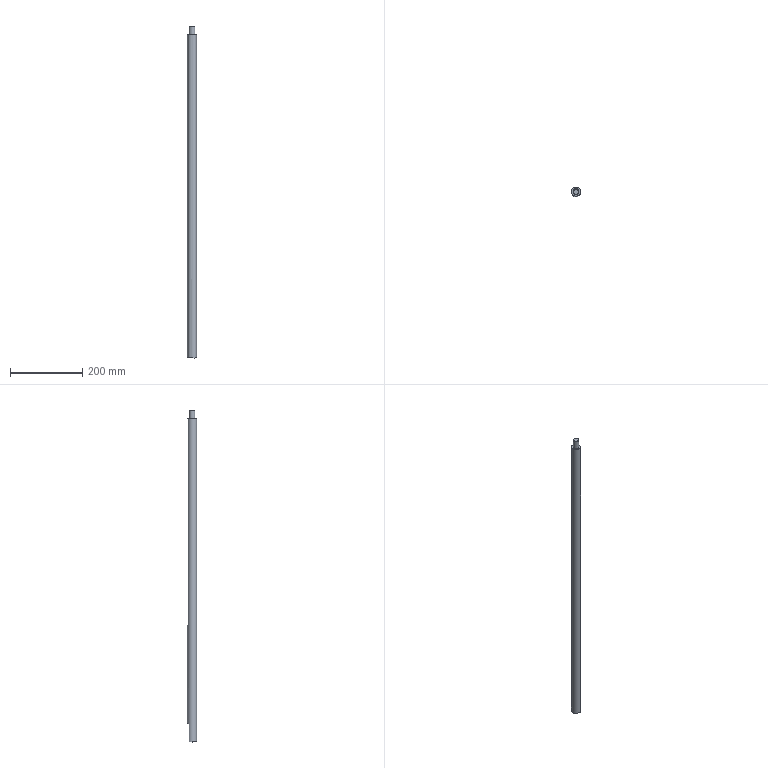Part | STEP file | solid 48 | 1 solid | 11 faces | box 25 x 25 x 917.392 mm | volume 438618 mm3 | plane 5 | cylinder 3 | cone 3 | commonest cylinder face diameters 10.2 x1 16 x1 25 x1